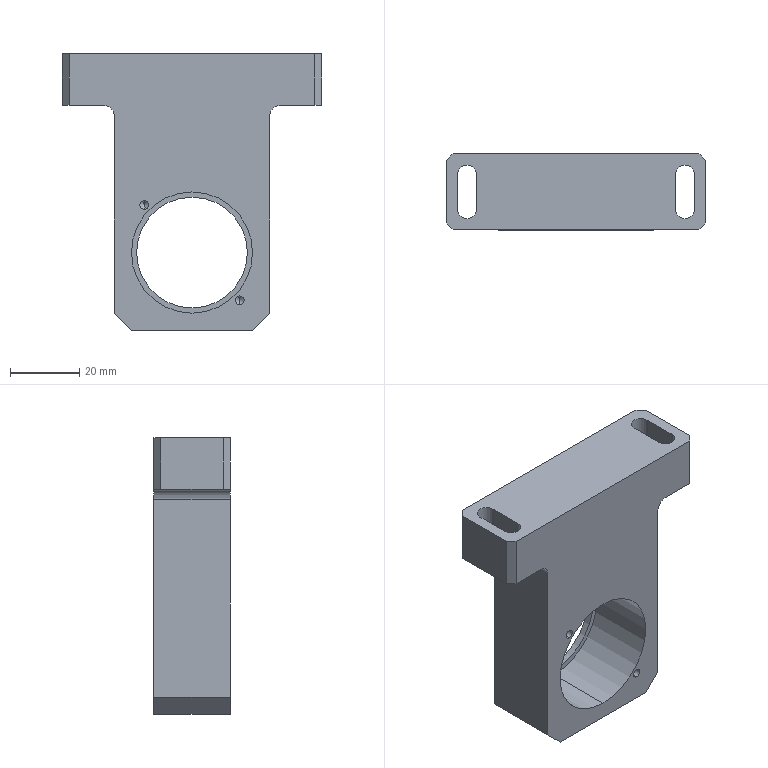Part | SolidWorks | features ICE 3, Chamfer 2, HoleWzd 2, CirPattern 1, Extrusion 1, Fillet 1 | 1 solid | 39 faces | box 75 x 22 x 80 mm | volume 65225 mm3 | plane 21 | cylinder 14 | cone 4 | commonest cylinder face diameters 2.5 x4 5.5 x4 6 x2 32 x2 35 x2
STEP:
#1=CARTESIAN_POINT('',(-13.789,-3.5,-2.461));
#2=VERTEX_POINT('',#1);
#3=CARTESIAN_POINT('',(-13.789,-3.5,-4.961));
#4=VERTEX_POINT('',#3);
#5=CARTESIAN_POINT('',(-13.789,-3.5,-3.711));
#6=DIRECTION('',(0.,-1.,0.));
#7=DIRECTION('',(0.,0.,-1.));
#8=AXIS2_PLACEMENT_3D('',#5,#6,#7);
#9=CIRCLE('',#8,1.25);
#10=EDGE_CURVE('',#2,#4,#9,.T.);
#11=ORIENTED_EDGE('',*,*,#10,.F.);
#12=CARTESIAN_POINT('',(-13.789,-11.,-2.461));
#13=VERTEX_POINT('',#12);
#14=CARTESIAN_POINT('',(-13.789,-11.,-2.461));
#15=DIRECTION('',(0.,-1.,0.));
#16=VECTOR('',#15,1000.);
#17=LINE('',#14,#16);
#18=EDGE_CURVE('',#2,#13,#17,.T.);
#19=ORIENTED_EDGE('',*,*,#18,.T.);
#20=CARTESIAN_POINT('',(-13.789,-11.,-4.961));
#21=VERTEX_POINT('',#20);
#22=CARTESIAN_POINT('',(-13.789,-11.,-3.711));
#23=DIRECTION('',(0.,-1.,0.));
#24=DIRECTION('',(0.,0.,-1.));
#25=AXIS2_PLACEMENT_3D('',#22,#23,#24);
#26=CIRCLE('',#25,1.25);
#27=EDGE_CURVE('',#13,#21,#26,.T.);
#28=ORIENTED_EDGE('',*,*,#27,.T.);
#29=CARTESIAN_POINT('',(-13.789,-11.,-4.961));
#30=DIRECTION('',(0.,-1.,0.));
#31=VECTOR('',#30,1000.);
#32=LINE('',#29,#31);
#33=EDGE_CURVE('',#4,#21,#32,.T.);
#34=ORIENTED_EDGE('',*,*,#33,.F.);
#35=EDGE_LOOP('',(#11,#19,#28,#34));
#36=FACE_OUTER_BOUND('',#35,.T.);
#37=CARTESIAN_POINT('',(-13.789,-11.,-3.711));
#38=DIRECTION('',(0.,-1.,0.));
#39=DIRECTION('',(0.,0.,-1.));
#40=AXIS2_PLACEMENT_3D('',#37,#38,#39);
#41=CYLINDRICAL_SURFACE('',#40,1.25);
#42=ADVANCED_FACE('',(#36),#41,.F.);
#43=CARTESIAN_POINT('',(-13.789,-2.749,-3.711));
#44=VERTEX_POINT('',#43);
#45=CARTESIAN_POINT('',(-13.789,-3.5,-4.961));
#46=DIRECTION('',(0.,-0.515,-0.8572));
#47=VECTOR('',#46,1000.);
#48=LINE('',#45,#47);
#49=EDGE_CURVE('',#44,#4,#48,.T.);
#50=ORIENTED_EDGE('',*,*,#49,.F.);
#51=CARTESIAN_POINT('',(-13.789,-3.5,-2.461));
#52=DIRECTION('',(0.,-0.515,0.8572));
#53=VECTOR('',#52,1000.);
#54=LINE('',#51,#53);
#55=EDGE_CURVE('',#44,#2,#54,.T.);
#56=ORIENTED_EDGE('',*,*,#55,.T.);
#57=ORIENTED_EDGE('',*,*,#10,.T.);
#58=EDGE_LOOP('',(#50,#56,#57));
#59=FACE_OUTER_BOUND('',#58,.T.);
#60=CARTESIAN_POINT('',(-13.789,-3.5,-3.711));
#61=DIRECTION('',(0.,-1.,0.));
#62=DIRECTION('',(0.,0.,-1.));
#63=AXIS2_PLACEMENT_3D('',#60,#61,#62);
#64=CONICAL_SURFACE('',#63,1.25,1.03);
#65=ADVANCED_FACE('',(#59),#64,.F.);
#66=CARTESIAN_POINT('',(13.789,-3.5,-30.039));
#67=VERTEX_POINT('',#66);
#68=CARTESIAN_POINT('',(13.789,-3.5,-32.539));
#69=VERTEX_POINT('',#68);
#70=CARTESIAN_POINT('',(13.789,-3.5,-31.289));
#71=DIRECTION('',(0.,-1.,0.));
#72=DIRECTION('',(0.,0.,-1.));
#73=AXIS2_PLACEMENT_3D('',#70,#71,#72);
#74=CIRCLE('',#73,1.25);
#75=EDGE_CURVE('',#67,#69,#74,.T.);
#76=ORIENTED_EDGE('',*,*,#75,.F.);
#77=CARTESIAN_POINT('',(13.789,-11.,-30.039));
#78=VERTEX_POINT('',#77);
#79=CARTESIAN_POINT('',(13.789,-11.,-30.039));
#80=DIRECTION('',(0.,-1.,0.));
#81=VECTOR('',#80,1000.);
#82=LINE('',#79,#81);
#83=EDGE_CURVE('',#67,#78,#82,.T.);
#84=ORIENTED_EDGE('',*,*,#83,.T.);
#85=CARTESIAN_POINT('',(13.789,-11.,-32.539));
#86=VERTEX_POINT('',#85);
#87=CARTESIAN_POINT('',(13.789,-11.,-31.289));
#88=DIRECTION('',(0.,-1.,0.));
#89=DIRECTION('',(0.,0.,-1.));
#90=AXIS2_PLACEMENT_3D('',#87,#88,#89);
#91=CIRCLE('',#90,1.25);
#92=EDGE_CURVE('',#78,#86,#91,.T.);
#93=ORIENTED_EDGE('',*,*,#92,.T.);
#94=CARTESIAN_POINT('',(13.789,-11.,-32.539));
#95=DIRECTION('',(0.,-1.,0.));
#96=VECTOR('',#95,1000.);
#97=LINE('',#94,#96);
#98=EDGE_CURVE('',#69,#86,#97,.T.);
#99=ORIENTED_EDGE('',*,*,#98,.F.);
#100=EDGE_LOOP('',(#76,#84,#93,#99));
#101=FACE_OUTER_BOUND('',#100,.T.);
#102=CARTESIAN_POINT('',(13.789,-11.,-31.289));
#103=DIRECTION('',(0.,-1.,0.));
#104=DIRECTION('',(0.,0.,-1.));
#105=AXIS2_PLACEMENT_3D('',#102,#103,#104);
#106=CYLINDRICAL_SURFACE('',#105,1.25);
#107=ADVANCED_FACE('',(#101),#106,.F.);
#108=CARTESIAN_POINT('',(13.789,-2.749,-31.289));
#109=VERTEX_POINT('',#108);
#110=CARTESIAN_POINT('',(13.789,-3.5,-32.539));
#111=DIRECTION('',(0.,-0.515,-0.8572));
#112=VECTOR('',#111,1000.);
#113=LINE('',#110,#112);
#114=EDGE_CURVE('',#109,#69,#113,.T.);
#115=ORIENTED_EDGE('',*,*,#114,.F.);
#116=CARTESIAN_POINT('',(13.789,-3.5,-30.039));
#117=DIRECTION('',(0.,-0.515,0.8572));
#118=VECTOR('',#117,1000.);
#119=LINE('',#116,#118);
#120=EDGE_CURVE('',#109,#67,#119,.T.);
#121=ORIENTED_EDGE('',*,*,#120,.T.);
#122=ORIENTED_EDGE('',*,*,#75,.T.);
#123=EDGE_LOOP('',(#115,#121,#122));
#124=FACE_OUTER_BOUND('',#123,.T.);
#125=CARTESIAN_POINT('',(13.789,-3.5,-31.289));
#126=DIRECTION('',(0.,-1.,0.));
#127=DIRECTION('',(0.,0.,-1.));
#128=AXIS2_PLACEMENT_3D('',#125,#126,#127);
#129=CONICAL_SURFACE('',#128,1.25,1.03);
#130=ADVANCED_FACE('',(#124),#129,.F.);
#131=CARTESIAN_POINT('',(0.,9.,-33.5));
#132=VERTEX_POINT('',#131);
#133=CARTESIAN_POINT('',(0.,9.,-1.5));
#134=VERTEX_POINT('',#133);
#135=CARTESIAN_POINT('',(0.,9.,-17.5));
#136=DIRECTION('',(0.,1.,0.));
#137=DIRECTION('',(0.,0.,1.));
#138=AXIS2_PLACEMENT_3D('',#135,#136,#137);
#139=CIRCLE('',#138,16.);
#140=EDGE_CURVE('',#132,#134,#139,.T.);
#141=ORIENTED_EDGE('',*,*,#140,.F.);
#142=CARTESIAN_POINT('',(0.,11.,-33.5));
#143=VERTEX_POINT('',#142);
#144=CARTESIAN_POINT('',(0.,9.,-33.5));
#145=DIRECTION('',(0.,1.,0.));
#146=VECTOR('',#145,1000.);
#147=LINE('',#144,#146);
#148=EDGE_CURVE('',#132,#143,#147,.T.);
#149=ORIENTED_EDGE('',*,*,#148,.T.);
#150=CARTESIAN_POINT('',(0.,11.,-1.5));
#151=VERTEX_POINT('',#150);
#152=CARTESIAN_POINT('',(0.,11.,-17.5));
#153=DIRECTION('',(0.,1.,0.));
#154=DIRECTION('',(0.,0.,1.));
#155=AXIS2_PLACEMENT_3D('',#152,#153,#154);
#156=CIRCLE('',#155,16.);
#157=EDGE_CURVE('',#143,#151,#156,.T.);
#158=ORIENTED_EDGE('',*,*,#157,.T.);
#159=CARTESIAN_POINT('',(0.,9.,-1.5));
#160=DIRECTION('',(0.,1.,0.));
#161=VECTOR('',#160,1000.);
#162=LINE('',#159,#161);
#163=EDGE_CURVE('',#134,#151,#162,.T.);
#164=ORIENTED_EDGE('',*,*,#163,.F.);
#165=EDGE_LOOP('',(#141,#149,#158,#164));
#166=FACE_OUTER_BOUND('',#165,.T.);
#167=CARTESIAN_POINT('',(0.,9.,-17.5));
#168=DIRECTION('',(0.,1.,0.));
#169=DIRECTION('',(0.,0.,1.));
#170=AXIS2_PLACEMENT_3D('',#167,#168,#169);
#171=CYLINDRICAL_SURFACE('',#170,16.);
#172=ADVANCED_FACE('',(#166),#171,.F.);
#173=CARTESIAN_POINT('',(0.,-11.,-35.));
#174=VERTEX_POINT('',#173);
#175=CARTESIAN_POINT('',(0.,-11.,0.));
#176=VERTEX_POINT('',#175);
#177=CARTESIAN_POINT('',(0.,-11.,-17.5));
#178=DIRECTION('',(0.,1.,0.));
#179=DIRECTION('',(0.,0.,1.));
#180=AXIS2_PLACEMENT_3D('',#177,#178,#179);
#181=CIRCLE('',#180,17.5);
#182=EDGE_CURVE('',#174,#176,#181,.T.);
#183=ORIENTED_EDGE('',*,*,#182,.F.);
#184=CARTESIAN_POINT('',(0.,9.,-35.));
#185=VERTEX_POINT('',#184);
#186=CARTESIAN_POINT('',(0.,-11.,-35.));
#187=DIRECTION('',(0.,1.,0.));
#188=VECTOR('',#187,1000.);
#189=LINE('',#186,#188);
#190=EDGE_CURVE('',#174,#185,#189,.T.);
#191=ORIENTED_EDGE('',*,*,#190,.T.);
#192=CARTESIAN_POINT('',(0.,9.,0.));
#193=VERTEX_POINT('',#192);
#194=CARTESIAN_POINT('',(0.,9.,-17.5));
#195=DIRECTION('',(0.,-1.,0.));
#196=DIRECTION('',(0.,0.,1.));
#197=AXIS2_PLACEMENT_3D('',#194,#195,#196);
#198=CIRCLE('',#197,17.5);
#199=EDGE_CURVE('',#193,#185,#198,.T.);
#200=ORIENTED_EDGE('',*,*,#199,.F.);
#201=CARTESIAN_POINT('',(0.,-11.,0.));
#202=DIRECTION('',(0.,1.,0.));
#203=VECTOR('',#202,1000.);
#204=LINE('',#201,#203);
#205=EDGE_CURVE('',#176,#193,#204,.T.);
#206=ORIENTED_EDGE('',*,*,#205,.F.);
#207=EDGE_LOOP('',(#183,#191,#200,#206));
#208=FACE_OUTER_BOUND('',#207,.T.);
#209=CARTESIAN_POINT('',(0.,-11.,-17.5));
#210=DIRECTION('',(0.,1.,0.));
#211=DIRECTION('',(0.,0.,1.));
#212=AXIS2_PLACEMENT_3D('',#209,#210,#211);
#213=CYLINDRICAL_SURFACE('',#212,17.5);
#214=ADVANCED_FACE('',(#208),#213,.F.);
#215=ORIENTED_EDGE('',*,*,#190,.F.);
#216=CARTESIAN_POINT('',(0.,-11.,-17.5));
#217=DIRECTION('',(0.,1.,0.));
#218=DIRECTION('',(0.,0.,1.));
#219=AXIS2_PLACEMENT_3D('',#216,#217,#218);
#220=CIRCLE('',#219,17.5);
#221=EDGE_CURVE('',#176,#174,#220,.T.);
#222=ORIENTED_EDGE('',*,*,#221,.F.);
#223=ORIENTED_EDGE('',*,*,#205,.T.);
#224=CARTESIAN_POINT('',(0.,9.,-17.5));
#225=DIRECTION('',(0.,-1.,0.));
#226=DIRECTION('',(0.,0.,1.));
#227=AXIS2_PLACEMENT_3D('',#224,#225,#226);
#228=CIRCLE('',#227,17.5);
#229=EDGE_CURVE('',#185,#193,#228,.T.);
#230=ORIENTED_EDGE('',*,*,#229,.F.);
#231=EDGE_LOOP('',(#215,#222,#223,#230));
#232=FACE_OUTER_BOUND('',#231,.T.);
#233=CARTESIAN_POINT('',(0.,-11.,-17.5));
#234=DIRECTION('',(0.,1.,0.));
#235=DIRECTION('',(0.,0.,1.));
#236=AXIS2_PLACEMENT_3D('',#233,#234,#235);
#237=CYLINDRICAL_SURFACE('',#236,17.5);
#238=ADVANCED_FACE('',(#232),#237,.F.);
#239=CARTESIAN_POINT('',(22.5,-11.,22.));
#240=VERTEX_POINT('',#239);
#241=CARTESIAN_POINT('',(22.5,-11.,-35.));
#242=VERTEX_POINT('',#241);
#243=CARTESIAN_POINT('',(22.5,-11.,40.));
#244=DIRECTION('',(0.,0.,-1.));
#245=VECTOR('',#244,1000.);
#246=LINE('',#243,#245);
#247=EDGE_CURVE('',#240,#242,#246,.T.);
#248=ORIENTED_EDGE('',*,*,#247,.T.);
#249=CARTESIAN_POINT('',(22.5,11.,-35.));
#250=VERTEX_POINT('',#249);
#251=CARTESIAN_POINT('',(22.5,11.,-35.));
#252=DIRECTION('',(0.,1.,0.));
#253=VECTOR('',#252,1000.);
#254=LINE('',#251,#253);
#255=EDGE_CURVE('',#242,#250,#254,.T.);
#256=ORIENTED_EDGE('',*,*,#255,.T.);
#257=CARTESIAN_POINT('',(22.5,11.,22.));
#258=VERTEX_POINT('',#257);
#259=CARTESIAN_POINT('',(22.5,11.,40.));
#260=DIRECTION('',(0.,0.,-1.));
#261=VECTOR('',#260,1000.);
#262=LINE('',#259,#261);
#263=EDGE_CURVE('',#258,#250,#262,.T.);
#264=ORIENTED_EDGE('',*,*,#263,.F.);
#265=CARTESIAN_POINT('',(22.5,11.,22.));
#266=DIRECTION('',(0.,-1.,0.));
#267=VECTOR('',#266,1000.);
#268=LINE('',#265,#267);
#269=EDGE_CURVE('',#258,#240,#268,.T.);
#270=ORIENTED_EDGE('',*,*,#269,.T.);
#271=EDGE_LOOP('',(#248,#256,#264,#270));
#272=FACE_OUTER_BOUND('',#271,.T.);
#273=CARTESIAN_POINT('',(22.5,11.,40.));
#274=DIRECTION('',(-1.,0.,0.));
#275=DIRECTION('',(0.,0.,1.));
#276=AXIS2_PLACEMENT_3D('',#273,#274,#275);
#277=PLANE('',#276);
#278=ADVANCED_FACE('',(#272),#277,.F.);
#279=CARTESIAN_POINT('',(17.5,-11.,-40.));
#280=VERTEX_POINT('',#279);
#281=CARTESIAN_POINT('',(-17.5,-11.,-40.));
#282=VERTEX_POINT('',#281);
#283=CARTESIAN_POINT('',(-22.5,-11.,-40.));
#284=DIRECTION('',(-1.,0.,0.));
#285=VECTOR('',#284,1000.);
#286=LINE('',#283,#285);
#287=EDGE_CURVE('',#280,#282,#286,.T.);
#288=ORIENTED_EDGE('',*,*,#287,.T.);
#289=CARTESIAN_POINT('',(-17.5,11.,-40.));
#290=VERTEX_POINT('',#289);
#291=CARTESIAN_POINT('',(-17.5,11.,-40.));
#292=DIRECTION('',(0.,1.,0.));
#293=VECTOR('',#292,1000.);
#294=LINE('',#291,#293);
#295=EDGE_CURVE('',#282,#290,#294,.T.);
#296=ORIENTED_EDGE('',*,*,#295,.T.);
#297=CARTESIAN_POINT('',(17.5,11.,-40.));
#298=VERTEX_POINT('',#297);
#299=CARTESIAN_POINT('',(-22.5,11.,-40.));
#300=DIRECTION('',(-1.,0.,0.));
#301=VECTOR('',#300,1000.);
#302=LINE('',#299,#301);
#303=EDGE_CURVE('',#298,#290,#302,.T.);
#304=ORIENTED_EDGE('',*,*,#303,.F.);
#305=CARTESIAN_POINT('',(17.5,11.,-40.));
#306=DIRECTION('',(0.,-1.,0.));
#307=VECTOR('',#306,1000.);
#308=LINE('',#305,#307);
#309=EDGE_CURVE('',#298,#280,#308,.T.);
#310=ORIENTED_EDGE('',*,*,#309,.T.);
#311=EDGE_LOOP('',(#288,#296,#304,#310));
#312=FACE_OUTER_BOUND('',#311,.T.);
#313=CARTESIAN_POINT('',(-22.5,11.,-40.));
#314=DIRECTION('',(0.,0.,1.));
#315=DIRECTION('',(1.,0.,0.));
#316=AXIS2_PLACEMENT_3D('',#313,#314,#315);
#317=PLANE('',#316);
#318=ADVANCED_FACE('',(#312),#317,.F.);
#319=CARTESIAN_POINT('',(-22.5,11.,-35.));
#320=VERTEX_POINT('',#319);
#321=CARTESIAN_POINT('',(-22.5,11.,22.));
#322=VERTEX_POINT('',#321);
#323=CARTESIAN_POINT('',(-22.5,11.,40.));
#324=DIRECTION('',(0.,0.,1.));
#325=VECTOR('',#324,1000.);
#326=LINE('',#323,#325);
#327=EDGE_CURVE('',#320,#322,#326,.T.);
#328=ORIENTED_EDGE('',*,*,#327,.F.);
#329=CARTESIAN_POINT('',(-22.5,-11.,-35.));
#330=VERTEX_POINT('',#329);
#331=CARTESIAN_POINT('',(-22.5,11.,-35.));
#332=DIRECTION('',(0.,-1.,0.));
#333=VECTOR('',#332,1000.);
#334=LINE('',#331,#333);
#335=EDGE_CURVE('',#320,#330,#334,.T.);
#336=ORIENTED_EDGE('',*,*,#335,.T.);
#337=CARTESIAN_POINT('',(-22.5,-11.,22.));
#338=VERTEX_POINT('',#337);
#339=CARTESIAN_POINT('',(-22.5,-11.,40.));
#340=DIRECTION('',(0.,0.,1.));
#341=VECTOR('',#340,1000.);
#342=LINE('',#339,#341);
#343=EDGE_CURVE('',#330,#338,#342,.T.);
#344=ORIENTED_EDGE('',*,*,#343,.T.);
#345=CARTESIAN_POINT('',(-22.5,11.,22.));
#346=DIRECTION('',(0.,1.,0.));
#347=VECTOR('',#346,1000.);
#348=LINE('',#345,#347);
#349=EDGE_CURVE('',#338,#322,#348,.T.);
#350=ORIENTED_EDGE('',*,*,#349,.T.);
#351=EDGE_LOOP('',(#328,#336,#344,#350));
#352=FACE_OUTER_BOUND('',#351,.T.);
#353=CARTESIAN_POINT('',(-22.5,11.,40.));
#354=DIRECTION('',(1.,0.,0.));
#355=DIRECTION('',(0.,0.,-1.));
#356=AXIS2_PLACEMENT_3D('',#353,#354,#355);
#357=PLANE('',#356);
#358=ADVANCED_FACE('',(#352),#357,.F.);
#359=CARTESIAN_POINT('',(28.75,-5.,40.));
#360=VERTEX_POINT('',#359);
#361=CARTESIAN_POINT('',(28.75,5.,40.));
#362=VERTEX_POINT('',#361);
#363=CARTESIAN_POINT('',(28.75,-5.,40.));
#364=DIRECTION('',(0.,1.,0.));
#365=VECTOR('',#364,1000.);
#366=LINE('',#363,#365);
#367=EDGE_CURVE('',#360,#362,#366,.T.);
#368=ORIENTED_EDGE('',*,*,#367,.T.);
#369=CARTESIAN_POINT('',(34.25,5.,40.));
#370=VERTEX_POINT('',#369);
#371=CARTESIAN_POINT('',(31.5,5.,40.));
#372=DIRECTION('',(0.,0.,-1.));
#373=DIRECTION('',(-1.,0.,0.));
#374=AXIS2_PLACEMENT_3D('',#371,#372,#373);
#375=CIRCLE('',#374,2.75);
#376=EDGE_CURVE('',#362,#370,#375,.T.);
#377=ORIENTED_EDGE('',*,*,#376,.T.);
#378=CARTESIAN_POINT('',(34.25,-5.,40.));
#379=VERTEX_POINT('',#378);
#380=CARTESIAN_POINT('',(34.25,-5.,40.));
#381=DIRECTION('',(0.,1.,0.));
#382=VECTOR('',#381,1000.);
#383=LINE('',#380,#382);
#384=EDGE_CURVE('',#379,#370,#383,.T.);
#385=ORIENTED_EDGE('',*,*,#384,.F.);
#386=CARTESIAN_POINT('',(31.5,-5.,40.));
#387=DIRECTION('',(0.,0.,-1.));
#388=DIRECTION('',(-1.,0.,0.));
#389=AXIS2_PLACEMENT_3D('',#386,#387,#388);
#390=CIRCLE('',#389,2.75);
#391=EDGE_CURVE('',#379,#360,#390,.T.);
#392=ORIENTED_EDGE('',*,*,#391,.T.);
#393=EDGE_LOOP('',(#368,#377,#385,#392));
#394=FACE_BOUND('',#393,.T.);
#395=CARTESIAN_POINT('',(-34.25,-5.,40.));
#396=VERTEX_POINT('',#395);
#397=CARTESIAN_POINT('',(-34.25,5.,40.));
#398=VERTEX_POINT('',#397);
#399=CARTESIAN_POINT('',(-34.25,-5.,40.));
#400=DIRECTION('',(0.,1.,0.));
#401=VECTOR('',#400,1000.);
#402=LINE('',#399,#401);
#403=EDGE_CURVE('',#396,#398,#402,.T.);
#404=ORIENTED_EDGE('',*,*,#403,.T.);
#405=CARTESIAN_POINT('',(-28.75,5.,40.));
#406=VERTEX_POINT('',#405);
#407=CARTESIAN_POINT('',(-31.5,5.,40.));
#408=DIRECTION('',(0.,0.,-1.));
#409=DIRECTION('',(-1.,0.,0.));
#410=AXIS2_PLACEMENT_3D('',#407,#408,#409);
#411=CIRCLE('',#410,2.75);
#412=EDGE_CURVE('',#398,#406,#411,.T.);
#413=ORIENTED_EDGE('',*,*,#412,.T.);
#414=CARTESIAN_POINT('',(-28.75,-5.,40.));
#415=VERTEX_POINT('',#414);
#416=CARTESIAN_POINT('',(-28.75,-5.,40.));
#417=DIRECTION('',(0.,1.,0.));
#418=VECTOR('',#417,1000.);
#419=LINE('',#416,#418);
#420=EDGE_CURVE('',#415,#406,#419,.T.);
#421=ORIENTED_EDGE('',*,*,#420,.F.);
#422=CARTESIAN_POINT('',(-31.5,-5.,40.));
#423=DIRECTION('',(0.,0.,-1.));
#424=DIRECTION('',(-1.,0.,0.));
#425=AXIS2_PLACEMENT_3D('',#422,#423,#424);
#426=CIRCLE('',#425,2.75);
#427=EDGE_CURVE('',#415,#396,#426,.T.);
#428=ORIENTED_EDGE('',*,*,#427,.T.);
#429=EDGE_LOOP('',(#404,#413,#421,#428));
#430=FACE_BOUND('',#429,.T.);
#431=CARTESIAN_POINT('',(-37.5,-9.,40.));
#432=VERTEX_POINT('',#431);
#433=CARTESIAN_POINT('',(-37.5,9.,40.));
#434=VERTEX_POINT('',#433);
#435=CARTESIAN_POINT('',(-37.5,-32.213,40.));
#436=DIRECTION('',(0.,1.,0.));
#437=VECTOR('',#436,1000.);
#438=LINE('',#435,#437);
#439=EDGE_CURVE('',#432,#434,#438,.T.);
#440=ORIENTED_EDGE('',*,*,#439,.F.);
#441=CARTESIAN_POINT('',(-35.5,-11.,40.));
#442=VERTEX_POINT('',#441);
#443=CARTESIAN_POINT('',(-37.5,-9.,40.));
#444=DIRECTION('',(0.7071,-0.7071,0.));
#445=VECTOR('',#444,1000.);
#446=LINE('',#443,#445);
#447=EDGE_CURVE('',#432,#442,#446,.T.);
#448=ORIENTED_EDGE('',*,*,#447,.T.);
#449=CARTESIAN_POINT('',(35.5,-11.,40.));
#450=VERTEX_POINT('',#449);
#451=CARTESIAN_POINT('',(-22.5,-11.,40.));
#452=DIRECTION('',(1.,0.,0.));
#453=VECTOR('',#452,1000.);
#454=LINE('',#451,#453);
#455=EDGE_CURVE('',#442,#450,#454,.T.);
#456=ORIENTED_EDGE('',*,*,#455,.T.);
#457=CARTESIAN_POINT('',(37.5,-9.,40.));
#458=VERTEX_POINT('',#457);
#459=CARTESIAN_POINT('',(37.5,-9.,40.));
#460=DIRECTION('',(0.7071,0.7071,0.));
#461=VECTOR('',#460,1000.);
#462=LINE('',#459,#461);
#463=EDGE_CURVE('',#450,#458,#462,.T.);
#464=ORIENTED_EDGE('',*,*,#463,.T.);
#465=CARTESIAN_POINT('',(37.5,9.,40.));
#466=VERTEX_POINT('',#465);
#467=CARTESIAN_POINT('',(37.5,-32.213,40.));
#468=DIRECTION('',(0.,1.,0.));
#469=VECTOR('',#468,1000.);
#470=LINE('',#467,#469);
#471=EDGE_CURVE('',#458,#466,#470,.T.);
#472=ORIENTED_EDGE('',*,*,#471,.T.);
#473=CARTESIAN_POINT('',(35.5,11.,40.));
#474=VERTEX_POINT('',#473);
#475=CARTESIAN_POINT('',(35.5,11.,40.));
#476=DIRECTION('',(-0.7071,0.7071,0.));
#477=VECTOR('',#476,1000.);
#478=LINE('',#475,#477);
#479=EDGE_CURVE('',#466,#474,#478,.T.);
#480=ORIENTED_EDGE('',*,*,#479,.T.);
#481=CARTESIAN_POINT('',(-35.5,11.,40.));
#482=VERTEX_POINT('',#481);
#483=CARTESIAN_POINT('',(-22.5,11.,40.));
#484=DIRECTION('',(1.,0.,0.));
#485=VECTOR('',#484,1000.);
#486=LINE('',#483,#485);
#487=EDGE_CURVE('',#482,#474,#486,.T.);
#488=ORIENTED_EDGE('',*,*,#487,.F.);
#489=CARTESIAN_POINT('',(-35.5,11.,40.));
#490=DIRECTION('',(-0.7071,-0.7071,0.));
#491=VECTOR('',#490,1000.);
#492=LINE('',#489,#491);
#493=EDGE_CURVE('',#482,#434,#492,.T.);
#494=ORIENTED_EDGE('',*,*,#493,.T.);
#495=EDGE_LOOP('',(#440,#448,#456,#464,#472,#480,#488,#494));
#496=FACE_OUTER_BOUND('',#495,.T.);
#497=CARTESIAN_POINT('',(-22.5,11.,40.));
#498=DIRECTION('',(0.,0.,-1.));
#499=DIRECTION('',(-1.,0.,0.));
#500=AXIS2_PLACEMENT_3D('',#497,#498,#499);
#501=PLANE('',#500);
#502=ADVANCED_FACE('',(#394,#430,#496),#501,.F.);
#503=CARTESIAN_POINT('',(-25.5,11.,25.));
#504=VERTEX_POINT('',#503);
#505=CARTESIAN_POINT('',(-35.5,11.,25.));
#506=VERTEX_POINT('',#505);
#507=CARTESIAN_POINT('',(-22.5,11.,25.));
#508=DIRECTION('',(-1.,0.,0.));
#509=VECTOR('',#508,1000.);
#510=LINE('',#507,#509);
#511=EDGE_CURVE('',#504,#506,#510,.T.);
#512=ORIENTED_EDGE('',*,*,#511,.T.);
#513=CARTESIAN_POINT('',(-35.5,11.,40.));
#514=DIRECTION('',(0.,0.,1.));
#515=VECTOR('',#514,1000.);
#516=LINE('',#513,#515);
#517=EDGE_CURVE('',#506,#482,#516,.T.);
#518=ORIENTED_EDGE('',*,*,#517,.T.);
#519=ORIENTED_EDGE('',*,*,#487,.T.);
#520=CARTESIAN_POINT('',(35.5,11.,25.));
#521=VERTEX_POINT('',#520);
#522=CARTESIAN_POINT('',(35.5,11.,25.));
#523=DIRECTION('',(0.,0.,-1.));
#524=VECTOR('',#523,1000.);
#525=LINE('',#522,#524);
#526=EDGE_CURVE('',#474,#521,#525,.T.);
#527=ORIENTED_EDGE('',*,*,#526,.T.);
#528=CARTESIAN_POINT('',(25.5,11.,25.));
#529=VERTEX_POINT('',#528);
#530=CARTESIAN_POINT('',(22.5,11.,25.));
#531=DIRECTION('',(-1.,0.,0.));
#532=VECTOR('',#531,1000.);
#533=LINE('',#530,#532);
#534=EDGE_CURVE('',#521,#529,#533,.T.);
#535=ORIENTED_EDGE('',*,*,#534,.T.);
#536=CARTESIAN_POINT('',(25.5,11.,22.));
#537=DIRECTION('',(0.,-1.,0.));
#538=DIRECTION('',(0.,0.,-1.));
#539=AXIS2_PLACEMENT_3D('',#536,#537,#538);
#540=CIRCLE('',#539,3.);
#541=EDGE_CURVE('',#529,#258,#540,.T.);
#542=ORIENTED_EDGE('',*,*,#541,.T.);
#543=ORIENTED_EDGE('',*,*,#263,.T.);
#544=CARTESIAN_POINT('',(17.5,11.,-40.));
#545=DIRECTION('',(-0.7071,0.,-0.7071));
#546=VECTOR('',#545,1000.);
#547=LINE('',#544,#546);
#548=EDGE_CURVE('',#250,#298,#547,.T.);
#549=ORIENTED_EDGE('',*,*,#548,.T.);
#550=ORIENTED_EDGE('',*,*,#303,.T.);
#551=CARTESIAN_POINT('',(-22.5,11.,-35.));
#552=DIRECTION('',(-0.7071,0.,0.7071));
#553=VECTOR('',#552,1000.);
#554=LINE('',#551,#553);
#555=EDGE_CURVE('',#290,#320,#554,.T.);
#556=ORIENTED_EDGE('',*,*,#555,.T.);
#557=ORIENTED_EDGE('',*,*,#327,.T.);
#558=CARTESIAN_POINT('',(-25.5,11.,22.));
#559=DIRECTION('',(0.,-1.,0.));
#560=DIRECTION('',(0.,0.,-1.));
#561=AXIS2_PLACEMENT_3D('',#558,#559,#560);
#562=CIRCLE('',#561,3.);
#563=EDGE_CURVE('',#322,#504,#562,.T.);
#564=ORIENTED_EDGE('',*,*,#563,.T.);
#565=EDGE_LOOP('',(#512,#518,#519,#527,#535,#542,#543,#549,#550,#556,#557,#564));
#566=FACE_OUTER_BOUND('',#565,.T.);
#567=CARTESIAN_POINT('',(0.,11.,-17.5));
#568=DIRECTION('',(0.,1.,0.));
#569=DIRECTION('',(0.,0.,1.));
#570=AXIS2_PLACEMENT_3D('',#567,#568,#569);
#571=CIRCLE('',#570,16.);
#572=EDGE_CURVE('',#151,#143,#571,.T.);
#573=ORIENTED_EDGE('',*,*,#572,.F.);
#574=ORIENTED_EDGE('',*,*,#157,.F.);
#575=EDGE_LOOP('',(#573,#574));
#576=FACE_BOUND('',#575,.T.);
#577=CARTESIAN_POINT('',(0.,11.,0.));
#578=DIRECTION('',(0.,-1.,0.));
#579=DIRECTION('',(0.,0.,-1.));
#580=AXIS2_PLACEMENT_3D('',#577,#578,#579);
#581=PLANE('',#580);
#582=ADVANCED_FACE('',(#566,#576),#581,.F.);
#583=CARTESIAN_POINT('',(-13.789,-11.,-3.711));
#584=DIRECTION('',(0.,-1.,0.));
#585=DIRECTION('',(0.,0.,-1.));
#586=AXIS2_PLACEMENT_3D('',#583,#584,#585);
#587=CIRCLE('',#586,1.25);
#588=EDGE_CURVE('',#21,#13,#587,.T.);
#589=ORIENTED_EDGE('',*,*,#588,.F.);
#590=ORIENTED_EDGE('',*,*,#27,.F.);
#591=EDGE_LOOP('',(#589,#590));
#592=FACE_BOUND('',#591,.T.);
#593=CARTESIAN_POINT('',(13.789,-11.,-31.289));
#594=DIRECTION('',(0.,-1.,0.));
#595=DIRECTION('',(0.,0.,-1.));
#596=AXIS2_PLACEMENT_3D('',#593,#594,#595);
#597=CIRCLE('',#596,1.25);
#598=EDGE_CURVE('',#86,#78,#597,.T.);
#599=ORIENTED_EDGE('',*,*,#598,.F.);
#600=ORIENTED_EDGE('',*,*,#92,.F.);
#601=EDGE_LOOP('',(#599,#600));
#602=FACE_BOUND('',#601,.T.);
#603=ORIENTED_EDGE('',*,*,#221,.T.);
#604=ORIENTED_EDGE('',*,*,#182,.T.);
#605=EDGE_LOOP('',(#603,#604));
#606=FACE_BOUND('',#605,.T.);
#607=ORIENTED_EDGE('',*,*,#455,.F.);
#608=CARTESIAN_POINT('',(-35.5,-11.,25.));
#609=VERTEX_POINT('',#608);
#610=CARTESIAN_POINT('',(-35.5,-11.,0.));
#611=DIRECTION('',(0.,0.,-1.));
#612=VECTOR('',#611,1000.);
#613=LINE('',#610,#612);
#614=EDGE_CURVE('',#442,#609,#613,.T.);
#615=ORIENTED_EDGE('',*,*,#614,.T.);
#616=CARTESIAN_POINT('',(-25.5,-11.,25.));
#617=VERTEX_POINT('',#616);
#618=CARTESIAN_POINT('',(-22.5,-11.,25.));
#619=DIRECTION('',(-1.,0.,0.));
#620=VECTOR('',#619,1000.);
#621=LINE('',#618,#620);
#622=EDGE_CURVE('',#617,#609,#621,.T.);
#623=ORIENTED_EDGE('',*,*,#622,.F.);
#624=CARTESIAN_POINT('',(-25.5,-11.,22.));
#625=DIRECTION('',(0.,1.,0.));
#626=DIRECTION('',(0.,0.,-1.));
#627=AXIS2_PLACEMENT_3D('',#624,#625,#626);
#628=CIRCLE('',#627,3.);
#629=EDGE_CURVE('',#617,#338,#628,.T.);
#630=ORIENTED_EDGE('',*,*,#629,.T.);
#631=ORIENTED_EDGE('',*,*,#343,.F.);
#632=CARTESIAN_POINT('',(-28.75,-11.,-28.75));
#633=DIRECTION('',(0.7071,0.,-0.7071));
#634=VECTOR('',#633,1000.);
#635=LINE('',#632,#634);
#636=EDGE_CURVE('',#330,#282,#635,.T.);
#637=ORIENTED_EDGE('',*,*,#636,.T.);
#638=ORIENTED_EDGE('',*,*,#287,.F.);
#639=CARTESIAN_POINT('',(28.75,-11.,-28.75));
#640=DIRECTION('',(0.7071,0.,0.7071));
#641=VECTOR('',#640,1000.);
#642=LINE('',#639,#641);
#643=EDGE_CURVE('',#280,#242,#642,.T.);
#644=ORIENTED_EDGE('',*,*,#643,.T.);
#645=ORIENTED_EDGE('',*,*,#247,.F.);
#646=CARTESIAN_POINT('',(25.5,-11.,25.));
#647=VERTEX_POINT('',#646);
#648=CARTESIAN_POINT('',(25.5,-11.,22.));
#649=DIRECTION('',(0.,1.,0.));
#650=DIRECTION('',(0.,0.,-1.));
#651=AXIS2_PLACEMENT_3D('',#648,#649,#650);
#652=CIRCLE('',#651,3.);
#653=EDGE_CURVE('',#240,#647,#652,.T.);
#654=ORIENTED_EDGE('',*,*,#653,.T.);
#655=CARTESIAN_POINT('',(35.5,-11.,25.));
#656=VERTEX_POINT('',#655);
#657=CARTESIAN_POINT('',(22.5,-11.,25.));
#658=DIRECTION('',(-1.,0.,0.));
#659=VECTOR('',#658,1000.);
#660=LINE('',#657,#659);
#661=EDGE_CURVE('',#656,#647,#660,.T.);
#662=ORIENTED_EDGE('',*,*,#661,.F.);
#663=CARTESIAN_POINT('',(35.5,-11.,0.));
#664=DIRECTION('',(0.,0.,1.));
#665=VECTOR('',#664,1000.);
#666=LINE('',#663,#665);
#667=EDGE_CURVE('',#656,#450,#666,.T.);
#668=ORIENTED_EDGE('',*,*,#667,.T.);
#669=EDGE_LOOP('',(#607,#615,#623,#630,#631,#637,#638,#644,#645,#654,#662,#668));
#670=FACE_OUTER_BOUND('',#669,.T.);
#671=CARTESIAN_POINT('',(0.,-11.,0.));
#672=DIRECTION('',(0.,-1.,0.));
#673=DIRECTION('',(0.,0.,-1.));
#674=AXIS2_PLACEMENT_3D('',#671,#672,#673);
#675=PLANE('',#674);
#676=ADVANCED_FACE('',(#592,#602,#606,#670),#675,.T.);
#677=CARTESIAN_POINT('',(-34.25,-5.,25.));
#678=VERTEX_POINT('',#677);
#679=CARTESIAN_POINT('',(-34.25,5.,25.));
#680=VERTEX_POINT('',#679);
#681=CARTESIAN_POINT('',(-34.25,-5.,25.));
#682=DIRECTION('',(0.,1.,0.));
#683=VECTOR('',#682,1000.);
#684=LINE('',#681,#683);
#685=EDGE_CURVE('',#678,#680,#684,.T.);
#686=ORIENTED_EDGE('',*,*,#685,.F.);
#687=CARTESIAN_POINT('',(-28.75,-5.,25.));
#688=VERTEX_POINT('',#687);
#689=CARTESIAN_POINT('',(-31.5,-5.,25.));
#690=DIRECTION('',(0.,0.,-1.));
#691=DIRECTION('',(-1.,0.,0.));
#692=AXIS2_PLACEMENT_3D('',#689,#690,#691);
#693=CIRCLE('',#692,2.75);
#694=EDGE_CURVE('',#688,#678,#693,.T.);
#695=ORIENTED_EDGE('',*,*,#694,.F.);
#696=CARTESIAN_POINT('',(-28.75,5.,25.));
#697=VERTEX_POINT('',#696);
#698=CARTESIAN_POINT('',(-28.75,-5.,25.));
#699=DIRECTION('',(0.,1.,0.));
#700=VECTOR('',#699,1000.);
#701=LINE('',#698,#700);
#702=EDGE_CURVE('',#688,#697,#701,.T.);
#703=ORIENTED_EDGE('',*,*,#702,.T.);
#704=CARTESIAN_POINT('',(-31.5,5.,25.));
#705=DIRECTION('',(0.,0.,-1.));
#706=DIRECTION('',(-1.,0.,0.));
#707=AXIS2_PLACEMENT_3D('',#704,#705,#706);
#708=CIRCLE('',#707,2.75);
#709=EDGE_CURVE('',#680,#697,#708,.T.);
#710=ORIENTED_EDGE('',*,*,#709,.F.);
#711=EDGE_LOOP('',(#686,#695,#703,#710));
#712=FACE_BOUND('',#711,.T.);
#713=ORIENTED_EDGE('',*,*,#622,.T.);
#714=CARTESIAN_POINT('',(-37.5,-9.,25.));
#715=VERTEX_POINT('',#714);
#716=CARTESIAN_POINT('',(-18.393,-28.107,25.));
#717=DIRECTION('',(-0.7071,0.7071,0.));
#718=VECTOR('',#717,1000.);
#719=LINE('',#716,#718);
#720=EDGE_CURVE('',#609,#715,#719,.T.);
#721=ORIENTED_EDGE('',*,*,#720,.T.);
#722=CARTESIAN_POINT('',(-37.5,9.,25.));
#723=VERTEX_POINT('',#722);
#724=CARTESIAN_POINT('',(-37.5,-32.213,25.));
#725=DIRECTION('',(0.,1.,0.));
#726=VECTOR('',#725,1000.);
#727=LINE('',#724,#726);
#728=EDGE_CURVE('',#715,#723,#727,.T.);
#729=ORIENTED_EDGE('',*,*,#728,.T.);
#730=CARTESIAN_POINT('',(-50.607,-4.107,25.));
#731=DIRECTION('',(0.7071,0.7071,0.));
#732=VECTOR('',#731,1000.);
#733=LINE('',#730,#732);
#734=EDGE_CURVE('',#723,#506,#733,.T.);
#735=ORIENTED_EDGE('',*,*,#734,.T.);
#736=ORIENTED_EDGE('',*,*,#511,.F.);
#737=CARTESIAN_POINT('',(-25.5,-32.213,25.));
#738=DIRECTION('',(0.,-1.,0.));
#739=VECTOR('',#738,1000.);
#740=LINE('',#737,#739);
#741=EDGE_CURVE('',#504,#617,#740,.T.);
#742=ORIENTED_EDGE('',*,*,#741,.T.);
#743=EDGE_LOOP('',(#713,#721,#729,#735,#736,#742));
#744=FACE_OUTER_BOUND('',#743,.T.);
#745=CARTESIAN_POINT('',(-22.5,-32.213,25.));
#746=DIRECTION('',(0.,0.,-1.));
#747=DIRECTION('',(-1.,0.,0.));
#748=AXIS2_PLACEMENT_3D('',#745,#746,#747);
#749=PLANE('',#748);
#750=ADVANCED_FACE('',(#712,#744),#749,.T.);
#751=ORIENTED_EDGE('',*,*,#728,.F.);
#752=CARTESIAN_POINT('',(-37.5,-9.,40.));
#753=DIRECTION('',(0.,0.,1.));
#754=VECTOR('',#753,1000.);
#755=LINE('',#752,#754);
#756=EDGE_CURVE('',#715,#432,#755,.T.);
#757=ORIENTED_EDGE('',*,*,#756,.T.);
#758=ORIENTED_EDGE('',*,*,#439,.T.);
#759=CARTESIAN_POINT('',(-37.5,9.,25.));
#760=DIRECTION('',(0.,0.,-1.));
#761=VECTOR('',#760,1000.);
#762=LINE('',#759,#761);
#763=EDGE_CURVE('',#434,#723,#762,.T.);
#764=ORIENTED_EDGE('',*,*,#763,.T.);
#765=EDGE_LOOP('',(#751,#757,#758,#764));
#766=FACE_OUTER_BOUND('',#765,.T.);
#767=CARTESIAN_POINT('',(-37.5,-32.213,40.));
#768=DIRECTION('',(-1.,0.,0.));
#769=DIRECTION('',(0.,0.,1.));
#770=AXIS2_PLACEMENT_3D('',#767,#768,#769);
#771=PLANE('',#770);
#772=ADVANCED_FACE('',(#766),#771,.T.);
#773=CARTESIAN_POINT('',(37.5,-9.,25.));
#774=VERTEX_POINT('',#773);
#775=CARTESIAN_POINT('',(37.5,9.,25.));
#776=VERTEX_POINT('',#775);
#777=CARTESIAN_POINT('',(37.5,-32.213,25.));
#778=DIRECTION('',(0.,1.,0.));
#779=VECTOR('',#778,1000.);
#780=LINE('',#777,#779);
#781=EDGE_CURVE('',#774,#776,#780,.T.);
#782=ORIENTED_EDGE('',*,*,#781,.T.);
#783=CARTESIAN_POINT('',(37.5,9.,40.));
#784=DIRECTION('',(0.,0.,1.));
#785=VECTOR('',#784,1000.);
#786=LINE('',#783,#785);
#787=EDGE_CURVE('',#776,#466,#786,.T.);
#788=ORIENTED_EDGE('',*,*,#787,.T.);
#789=ORIENTED_EDGE('',*,*,#471,.F.);
#790=CARTESIAN_POINT('',(37.5,-9.,40.));
#791=DIRECTION('',(0.,0.,-1.));
#792=VECTOR('',#791,1000.);
#793=LINE('',#790,#792);
#794=EDGE_CURVE('',#458,#774,#793,.T.);
#795=ORIENTED_EDGE('',*,*,#794,.T.);
#796=EDGE_LOOP('',(#782,#788,#789,#795));
#797=FACE_OUTER_BOUND('',#796,.T.);
#798=CARTESIAN_POINT('',(37.5,-32.213,40.));
#799=DIRECTION('',(1.,0.,0.));
#800=DIRECTION('',(0.,0.,-1.));
#801=AXIS2_PLACEMENT_3D('',#798,#799,#800);
#802=PLANE('',#801);
#803=ADVANCED_FACE('',(#797),#802,.T.);
#804=CARTESIAN_POINT('',(28.75,5.,25.));
#805=VERTEX_POINT('',#804);
#806=CARTESIAN_POINT('',(34.25,5.,25.));
#807=VERTEX_POINT('',#806);
#808=CARTESIAN_POINT('',(31.5,5.,25.));
#809=DIRECTION('',(0.,0.,-1.));
#810=DIRECTION('',(-1.,0.,0.));
#811=AXIS2_PLACEMENT_3D('',#808,#809,#810);
#812=CIRCLE('',#811,2.75);
#813=EDGE_CURVE('',#805,#807,#812,.T.);
#814=ORIENTED_EDGE('',*,*,#813,.F.);
#815=CARTESIAN_POINT('',(28.75,-5.,25.));
#816=VERTEX_POINT('',#815);
#817=CARTESIAN_POINT('',(28.75,-5.,25.));
#818=DIRECTION('',(0.,1.,0.));
#819=VECTOR('',#818,1000.);
#820=LINE('',#817,#819);
#821=EDGE_CURVE('',#816,#805,#820,.T.);
#822=ORIENTED_EDGE('',*,*,#821,.F.);
#823=CARTESIAN_POINT('',(34.25,-5.,25.));
#824=VERTEX_POINT('',#823);
#825=CARTESIAN_POINT('',(31.5,-5.,25.));
#826=DIRECTION('',(0.,0.,-1.));
#827=DIRECTION('',(-1.,0.,0.));
#828=AXIS2_PLACEMENT_3D('',#825,#826,#827);
#829=CIRCLE('',#828,2.75);
#830=EDGE_CURVE('',#824,#816,#829,.T.);
#831=ORIENTED_EDGE('',*,*,#830,.F.);
#832=CARTESIAN_POINT('',(34.25,-5.,25.));
#833=DIRECTION('',(0.,1.,0.));
#834=VECTOR('',#833,1000.);
#835=LINE('',#832,#834);
#836=EDGE_CURVE('',#824,#807,#835,.T.);
#837=ORIENTED_EDGE('',*,*,#836,.T.);
#838=EDGE_LOOP('',(#814,#822,#831,#837));
#839=FACE_BOUND('',#838,.T.);
#840=ORIENTED_EDGE('',*,*,#534,.F.);
#841=CARTESIAN_POINT('',(50.607,-4.107,25.));
#842=DIRECTION('',(0.7071,-0.7071,0.));
#843=VECTOR('',#842,1000.);
#844=LINE('',#841,#843);
#845=EDGE_CURVE('',#521,#776,#844,.T.);
#846=ORIENTED_EDGE('',*,*,#845,.T.);
#847=ORIENTED_EDGE('',*,*,#781,.F.);
#848=CARTESIAN_POINT('',(18.393,-28.107,25.));
#849=DIRECTION('',(-0.7071,-0.7071,0.));
#850=VECTOR('',#849,1000.);
#851=LINE('',#848,#850);
#852=EDGE_CURVE('',#774,#656,#851,.T.);
#853=ORIENTED_EDGE('',*,*,#852,.T.);
#854=ORIENTED_EDGE('',*,*,#661,.T.);
#855=CARTESIAN_POINT('',(25.5,-32.213,25.));
#856=DIRECTION('',(0.,1.,0.));
#857=VECTOR('',#856,1000.);
#858=LINE('',#855,#857);
#859=EDGE_CURVE('',#647,#529,#858,.T.);
#860=ORIENTED_EDGE('',*,*,#859,.T.);
#861=EDGE_LOOP('',(#840,#846,#847,#853,#854,#860));
#862=FACE_OUTER_BOUND('',#861,.T.);
#863=CARTESIAN_POINT('',(22.5,-32.213,25.));
#864=DIRECTION('',(0.,0.,-1.));
#865=DIRECTION('',(-1.,0.,0.));
#866=AXIS2_PLACEMENT_3D('',#863,#864,#865);
#867=PLANE('',#866);
#868=ADVANCED_FACE('',(#839,#862),#867,.T.);
#869=ORIENTED_EDGE('',*,*,#653,.F.);
#870=ORIENTED_EDGE('',*,*,#269,.F.);
#871=ORIENTED_EDGE('',*,*,#541,.F.);
#872=ORIENTED_EDGE('',*,*,#859,.F.);
#873=EDGE_LOOP('',(#869,#870,#871,#872));
#874=FACE_OUTER_BOUND('',#873,.T.);
#875=CARTESIAN_POINT('',(25.5,-32.213,22.));
#876=DIRECTION('',(0.,1.,0.));
#877=DIRECTION('',(0.,0.,1.));
#878=AXIS2_PLACEMENT_3D('',#875,#876,#877);
#879=CYLINDRICAL_SURFACE('',#878,3.);
#880=ADVANCED_FACE('',(#874),#879,.F.);
#881=ORIENTED_EDGE('',*,*,#629,.F.);
#882=ORIENTED_EDGE('',*,*,#741,.F.);
#883=ORIENTED_EDGE('',*,*,#563,.F.);
#884=ORIENTED_EDGE('',*,*,#349,.F.);
#885=EDGE_LOOP('',(#881,#882,#883,#884));
#886=FACE_OUTER_BOUND('',#885,.T.);
#887=CARTESIAN_POINT('',(-25.5,11.,22.));
#888=DIRECTION('',(0.,1.,0.));
#889=DIRECTION('',(0.,0.,1.));
#890=AXIS2_PLACEMENT_3D('',#887,#888,#889);
#891=CYLINDRICAL_SURFACE('',#890,3.);
#892=ADVANCED_FACE('',(#886),#891,.F.);
#893=ORIENTED_EDGE('',*,*,#555,.F.);
#894=ORIENTED_EDGE('',*,*,#295,.F.);
#895=ORIENTED_EDGE('',*,*,#636,.F.);
#896=ORIENTED_EDGE('',*,*,#335,.F.);
#897=EDGE_LOOP('',(#893,#894,#895,#896));
#898=FACE_OUTER_BOUND('',#897,.T.);
#899=CARTESIAN_POINT('',(-22.5,11.,-35.));
#900=DIRECTION('',(0.7071,0.,0.7071));
#901=DIRECTION('',(0.,-1.,0.));
#902=AXIS2_PLACEMENT_3D('',#899,#900,#901);
#903=PLANE('',#902);
#904=ADVANCED_FACE('',(#898),#903,.F.);
#905=ORIENTED_EDGE('',*,*,#548,.F.);
#906=ORIENTED_EDGE('',*,*,#255,.F.);
#907=ORIENTED_EDGE('',*,*,#643,.F.);
#908=ORIENTED_EDGE('',*,*,#309,.F.);
#909=EDGE_LOOP('',(#905,#906,#907,#908));
#910=FACE_OUTER_BOUND('',#909,.T.);
#911=CARTESIAN_POINT('',(17.5,11.,-40.));
#912=DIRECTION('',(-0.7071,0.,0.7071));
#913=DIRECTION('',(0.,-1.,0.));
#914=AXIS2_PLACEMENT_3D('',#911,#912,#913);
#915=PLANE('',#914);
#916=ADVANCED_FACE('',(#910),#915,.F.);
#917=CARTESIAN_POINT('',(0.,9.,-17.5));
#918=DIRECTION('',(0.,1.,0.));
#919=DIRECTION('',(0.,0.,1.));
#920=AXIS2_PLACEMENT_3D('',#917,#918,#919);
#921=CIRCLE('',#920,16.);
#922=EDGE_CURVE('',#134,#132,#921,.T.);
#923=ORIENTED_EDGE('',*,*,#922,.T.);
#924=ORIENTED_EDGE('',*,*,#140,.T.);
#925=EDGE_LOOP('',(#923,#924));
#926=FACE_BOUND('',#925,.T.);
#927=ORIENTED_EDGE('',*,*,#199,.T.);
#928=ORIENTED_EDGE('',*,*,#229,.T.);
#929=EDGE_LOOP('',(#927,#928));
#930=FACE_OUTER_BOUND('',#929,.T.);
#931=CARTESIAN_POINT('',(0.,9.,-17.5));
#932=DIRECTION('',(0.,1.,0.));
#933=DIRECTION('',(0.,0.,1.));
#934=AXIS2_PLACEMENT_3D('',#931,#932,#933);
#935=PLANE('',#934);
#936=ADVANCED_FACE('',(#926,#930),#935,.F.);
#937=ORIENTED_EDGE('',*,*,#148,.F.);
#938=ORIENTED_EDGE('',*,*,#922,.F.);
#939=ORIENTED_EDGE('',*,*,#163,.T.);
#940=ORIENTED_EDGE('',*,*,#572,.T.);
#941=EDGE_LOOP('',(#937,#938,#939,#940));
#942=FACE_OUTER_BOUND('',#941,.T.);
#943=CARTESIAN_POINT('',(0.,9.,-17.5));
#944=DIRECTION('',(0.,1.,0.));
#945=DIRECTION('',(0.,0.,1.));
#946=AXIS2_PLACEMENT_3D('',#943,#944,#945);
#947=CYLINDRICAL_SURFACE('',#946,16.);
#948=ADVANCED_FACE('',(#942),#947,.F.);
#949=ORIENTED_EDGE('',*,*,#709,.T.);
#950=CARTESIAN_POINT('',(-28.75,5.,40.));
#951=DIRECTION('',(0.,0.,1.));
#952=VECTOR('',#951,1000.);
#953=LINE('',#950,#952);
#954=EDGE_CURVE('',#697,#406,#953,.T.);
#955=ORIENTED_EDGE('',*,*,#954,.T.);
#956=ORIENTED_EDGE('',*,*,#412,.F.);
#957=CARTESIAN_POINT('',(-34.25,5.,25.));
#958=DIRECTION('',(0.,0.,1.));
#959=VECTOR('',#958,1000.);
#960=LINE('',#957,#959);
#961=EDGE_CURVE('',#680,#398,#960,.T.);
#962=ORIENTED_EDGE('',*,*,#961,.F.);
#963=EDGE_LOOP('',(#949,#955,#956,#962));
#964=FACE_OUTER_BOUND('',#963,.T.);
#965=CARTESIAN_POINT('',(-31.5,5.,25.));
#966=DIRECTION('',(0.,0.,-1.));
#967=DIRECTION('',(-1.,0.,0.));
#968=AXIS2_PLACEMENT_3D('',#965,#966,#967);
#969=CYLINDRICAL_SURFACE('',#968,2.75);
#970=ADVANCED_FACE('',(#964),#969,.F.);
#971=ORIENTED_EDGE('',*,*,#427,.F.);
#972=CARTESIAN_POINT('',(-28.75,-5.,40.));
#973=DIRECTION('',(0.,0.,1.));
#974=VECTOR('',#973,1000.);
#975=LINE('',#972,#974);
#976=EDGE_CURVE('',#688,#415,#975,.T.);
#977=ORIENTED_EDGE('',*,*,#976,.F.);
#978=ORIENTED_EDGE('',*,*,#694,.T.);
#979=CARTESIAN_POINT('',(-34.25,-5.,25.));
#980=DIRECTION('',(0.,0.,-1.));
#981=VECTOR('',#980,1000.);
#982=LINE('',#979,#981);
#983=EDGE_CURVE('',#396,#678,#982,.T.);
#984=ORIENTED_EDGE('',*,*,#983,.F.);
#985=EDGE_LOOP('',(#971,#977,#978,#984));
#986=FACE_OUTER_BOUND('',#985,.T.);
#987=CARTESIAN_POINT('',(-31.5,-5.,25.));
#988=DIRECTION('',(0.,0.,-1.));
#989=DIRECTION('',(-1.,0.,0.));
#990=AXIS2_PLACEMENT_3D('',#987,#988,#989);
#991=CYLINDRICAL_SURFACE('',#990,2.75);
#992=ADVANCED_FACE('',(#986),#991,.F.);
#993=ORIENTED_EDGE('',*,*,#954,.F.);
#994=ORIENTED_EDGE('',*,*,#702,.F.);
#995=ORIENTED_EDGE('',*,*,#976,.T.);
#996=ORIENTED_EDGE('',*,*,#420,.T.);
#997=EDGE_LOOP('',(#993,#994,#995,#996));
#998=FACE_OUTER_BOUND('',#997,.T.);
#999=CARTESIAN_POINT('',(-28.75,-5.,40.));
#1000=DIRECTION('',(-1.,0.,0.));
#1001=DIRECTION('',(0.,0.,1.));
#1002=AXIS2_PLACEMENT_3D('',#999,#1000,#1001);
#1003=PLANE('',#1002);
#1004=ADVANCED_FACE('',(#998),#1003,.T.);
#1005=ORIENTED_EDGE('',*,*,#961,.T.);
#1006=ORIENTED_EDGE('',*,*,#403,.F.);
#1007=ORIENTED_EDGE('',*,*,#983,.T.);
#1008=ORIENTED_EDGE('',*,*,#685,.T.);
#1009=EDGE_LOOP('',(#1005,#1006,#1007,#1008));
#1010=FACE_OUTER_BOUND('',#1009,.T.);
#1011=CARTESIAN_POINT('',(-34.25,-5.,25.));
#1012=DIRECTION('',(-1.,0.,0.));
#1013=DIRECTION('',(0.,0.,1.));
#1014=AXIS2_PLACEMENT_3D('',#1011,#1012,#1013);
#1015=PLANE('',#1014);
#1016=ADVANCED_FACE('',(#1010),#1015,.F.);
#1017=ORIENTED_EDGE('',*,*,#813,.T.);
#1018=CARTESIAN_POINT('',(34.25,5.,40.));
#1019=DIRECTION('',(0.,0.,1.));
#1020=VECTOR('',#1019,1000.);
#1021=LINE('',#1018,#1020);
#1022=EDGE_CURVE('',#807,#370,#1021,.T.);
#1023=ORIENTED_EDGE('',*,*,#1022,.T.);
#1024=ORIENTED_EDGE('',*,*,#376,.F.);
#1025=CARTESIAN_POINT('',(28.75,5.,25.));
#1026=DIRECTION('',(0.,0.,1.));
#1027=VECTOR('',#1026,1000.);
#1028=LINE('',#1025,#1027);
#1029=EDGE_CURVE('',#805,#362,#1028,.T.);
#1030=ORIENTED_EDGE('',*,*,#1029,.F.);
#1031=EDGE_LOOP('',(#1017,#1023,#1024,#1030));
#1032=FACE_OUTER_BOUND('',#1031,.T.);
#1033=CARTESIAN_POINT('',(31.5,5.,25.));
#1034=DIRECTION('',(0.,0.,-1.));
#1035=DIRECTION('',(-1.,0.,0.));
#1036=AXIS2_PLACEMENT_3D('',#1033,#1034,#1035);
#1037=CYLINDRICAL_SURFACE('',#1036,2.75);
#1038=ADVANCED_FACE('',(#1032),#1037,.F.);
#1039=ORIENTED_EDGE('',*,*,#391,.F.);
#1040=CARTESIAN_POINT('',(34.25,-5.,40.));
#1041=DIRECTION('',(0.,0.,1.));
#1042=VECTOR('',#1041,1000.);
#1043=LINE('',#1040,#1042);
#1044=EDGE_CURVE('',#824,#379,#1043,.T.);
#1045=ORIENTED_EDGE('',*,*,#1044,.F.);
#1046=ORIENTED_EDGE('',*,*,#830,.T.);
#1047=CARTESIAN_POINT('',(28.75,-5.,25.));
#1048=DIRECTION('',(0.,0.,-1.));
#1049=VECTOR('',#1048,1000.);
#1050=LINE('',#1047,#1049);
#1051=EDGE_CURVE('',#360,#816,#1050,.T.);
#1052=ORIENTED_EDGE('',*,*,#1051,.F.);
#1053=EDGE_LOOP('',(#1039,#1045,#1046,#1052));
#1054=FACE_OUTER_BOUND('',#1053,.T.);
#1055=CARTESIAN_POINT('',(31.5,-5.,25.));
#1056=DIRECTION('',(0.,0.,-1.));
#1057=DIRECTION('',(-1.,0.,0.));
#1058=AXIS2_PLACEMENT_3D('',#1055,#1056,#1057);
#1059=CYLINDRICAL_SURFACE('',#1058,2.75);
#1060=ADVANCED_FACE('',(#1054),#1059,.F.);
#1061=ORIENTED_EDGE('',*,*,#1022,.F.);
#1062=ORIENTED_EDGE('',*,*,#836,.F.);
#1063=ORIENTED_EDGE('',*,*,#1044,.T.);
#1064=ORIENTED_EDGE('',*,*,#384,.T.);
#1065=EDGE_LOOP('',(#1061,#1062,#1063,#1064));
#1066=FACE_OUTER_BOUND('',#1065,.T.);
#1067=CARTESIAN_POINT('',(34.25,-5.,40.));
#1068=DIRECTION('',(-1.,0.,0.));
#1069=DIRECTION('',(0.,0.,1.));
#1070=AXIS2_PLACEMENT_3D('',#1067,#1068,#1069);
#1071=PLANE('',#1070);
#1072=ADVANCED_FACE('',(#1066),#1071,.T.);
#1073=ORIENTED_EDGE('',*,*,#1029,.T.);
#1074=ORIENTED_EDGE('',*,*,#367,.F.);
#1075=ORIENTED_EDGE('',*,*,#1051,.T.);
#1076=ORIENTED_EDGE('',*,*,#821,.T.);
#1077=EDGE_LOOP('',(#1073,#1074,#1075,#1076));
#1078=FACE_OUTER_BOUND('',#1077,.T.);
#1079=CARTESIAN_POINT('',(28.75,-5.,25.));
#1080=DIRECTION('',(-1.,0.,0.));
#1081=DIRECTION('',(0.,0.,1.));
#1082=AXIS2_PLACEMENT_3D('',#1079,#1080,#1081);
#1083=PLANE('',#1082);
#1084=ADVANCED_FACE('',(#1078),#1083,.F.);
#1085=ORIENTED_EDGE('',*,*,#720,.F.);
#1086=ORIENTED_EDGE('',*,*,#614,.F.);
#1087=ORIENTED_EDGE('',*,*,#447,.F.);
#1088=ORIENTED_EDGE('',*,*,#756,.F.);
#1089=EDGE_LOOP('',(#1085,#1086,#1087,#1088));
#1090=FACE_OUTER_BOUND('',#1089,.T.);
#1091=CARTESIAN_POINT('',(-37.5,-9.,40.));
#1092=DIRECTION('',(0.7071,0.7071,0.));
#1093=DIRECTION('',(0.,0.,1.));
#1094=AXIS2_PLACEMENT_3D('',#1091,#1092,#1093);
#1095=PLANE('',#1094);
#1096=ADVANCED_FACE('',(#1090),#1095,.F.);
#1097=ORIENTED_EDGE('',*,*,#734,.F.);
#1098=ORIENTED_EDGE('',*,*,#763,.F.);
#1099=ORIENTED_EDGE('',*,*,#493,.F.);
#1100=ORIENTED_EDGE('',*,*,#517,.F.);
#1101=EDGE_LOOP('',(#1097,#1098,#1099,#1100));
#1102=FACE_OUTER_BOUND('',#1101,.T.);
#1103=CARTESIAN_POINT('',(-35.5,11.,0.));
#1104=DIRECTION('',(-0.7071,0.7071,0.));
#1105=DIRECTION('',(0.,0.,-1.));
#1106=AXIS2_PLACEMENT_3D('',#1103,#1104,#1105);
#1107=PLANE('',#1106);
#1108=ADVANCED_FACE('',(#1102),#1107,.T.);
#1109=ORIENTED_EDGE('',*,*,#479,.F.);
#1110=ORIENTED_EDGE('',*,*,#787,.F.);
#1111=ORIENTED_EDGE('',*,*,#845,.F.);
#1112=ORIENTED_EDGE('',*,*,#526,.F.);
#1113=EDGE_LOOP('',(#1109,#1110,#1111,#1112));
#1114=FACE_OUTER_BOUND('',#1113,.T.);
#1115=CARTESIAN_POINT('',(35.5,11.,0.));
#1116=DIRECTION('',(0.7071,0.7071,0.));
#1117=DIRECTION('',(0.,0.,1.));
#1118=AXIS2_PLACEMENT_3D('',#1115,#1116,#1117);
#1119=PLANE('',#1118);
#1120=ADVANCED_FACE('',(#1114),#1119,.T.);
#1121=ORIENTED_EDGE('',*,*,#463,.F.);
#1122=ORIENTED_EDGE('',*,*,#667,.F.);
#1123=ORIENTED_EDGE('',*,*,#852,.F.);
#1124=ORIENTED_EDGE('',*,*,#794,.F.);
#1125=EDGE_LOOP('',(#1121,#1122,#1123,#1124));
#1126=FACE_OUTER_BOUND('',#1125,.T.);
#1127=CARTESIAN_POINT('',(37.5,-9.,40.));
#1128=DIRECTION('',(-0.7071,0.7071,0.));
#1129=DIRECTION('',(0.,0.,-1.));
#1130=AXIS2_PLACEMENT_3D('',#1127,#1128,#1129);
#1131=PLANE('',#1130);
#1132=ADVANCED_FACE('',(#1126),#1131,.F.);
#1133=ORIENTED_EDGE('',*,*,#120,.F.);
#1134=ORIENTED_EDGE('',*,*,#114,.T.);
#1135=CARTESIAN_POINT('',(13.789,-3.5,-31.289));
#1136=DIRECTION('',(0.,-1.,0.));
#1137=DIRECTION('',(0.,0.,-1.));
#1138=AXIS2_PLACEMENT_3D('',#1135,#1136,#1137);
#1139=CIRCLE('',#1138,1.25);
#1140=EDGE_CURVE('',#69,#67,#1139,.T.);
#1141=ORIENTED_EDGE('',*,*,#1140,.T.);
#1142=EDGE_LOOP('',(#1133,#1134,#1141));
#1143=FACE_OUTER_BOUND('',#1142,.T.);
#1144=CARTESIAN_POINT('',(13.789,-3.5,-31.289));
#1145=DIRECTION('',(0.,-1.,0.));
#1146=DIRECTION('',(0.,0.,-1.));
#1147=AXIS2_PLACEMENT_3D('',#1144,#1145,#1146);
#1148=CONICAL_SURFACE('',#1147,1.25,1.03);
#1149=ADVANCED_FACE('',(#1143),#1148,.F.);
#1150=ORIENTED_EDGE('',*,*,#83,.F.);
#1151=ORIENTED_EDGE('',*,*,#1140,.F.);
#1152=ORIENTED_EDGE('',*,*,#98,.T.);
#1153=ORIENTED_EDGE('',*,*,#598,.T.);
#1154=EDGE_LOOP('',(#1150,#1151,#1152,#1153));
#1155=FACE_OUTER_BOUND('',#1154,.T.);
#1156=CARTESIAN_POINT('',(13.789,-11.,-31.289));
#1157=DIRECTION('',(0.,-1.,0.));
#1158=DIRECTION('',(0.,0.,-1.));
#1159=AXIS2_PLACEMENT_3D('',#1156,#1157,#1158);
#1160=CYLINDRICAL_SURFACE('',#1159,1.25);
#1161=ADVANCED_FACE('',(#1155),#1160,.F.);
#1162=ORIENTED_EDGE('',*,*,#55,.F.);
#1163=ORIENTED_EDGE('',*,*,#49,.T.);
#1164=CARTESIAN_POINT('',(-13.789,-3.5,-3.711));
#1165=DIRECTION('',(0.,-1.,0.));
#1166=DIRECTION('',(0.,0.,-1.));
#1167=AXIS2_PLACEMENT_3D('',#1164,#1165,#1166);
#1168=CIRCLE('',#1167,1.25);
#1169=EDGE_CURVE('',#4,#2,#1168,.T.);
#1170=ORIENTED_EDGE('',*,*,#1169,.T.);
#1171=EDGE_LOOP('',(#1162,#1163,#1170));
#1172=FACE_OUTER_BOUND('',#1171,.T.);
#1173=CARTESIAN_POINT('',(-13.789,-3.5,-3.711));
#1174=DIRECTION('',(0.,-1.,0.));
#1175=DIRECTION('',(0.,0.,-1.));
#1176=AXIS2_PLACEMENT_3D('',#1173,#1174,#1175);
#1177=CONICAL_SURFACE('',#1176,1.25,1.03);
#1178=ADVANCED_FACE('',(#1172),#1177,.F.);
#1179=ORIENTED_EDGE('',*,*,#18,.F.);
#1180=ORIENTED_EDGE('',*,*,#1169,.F.);
#1181=ORIENTED_EDGE('',*,*,#33,.T.);
#1182=ORIENTED_EDGE('',*,*,#588,.T.);
#1183=EDGE_LOOP('',(#1179,#1180,#1181,#1182));
#1184=FACE_OUTER_BOUND('',#1183,.T.);
#1185=CARTESIAN_POINT('',(-13.789,-11.,-3.711));
#1186=DIRECTION('',(0.,-1.,0.));
#1187=DIRECTION('',(0.,0.,-1.));
#1188=AXIS2_PLACEMENT_3D('',#1185,#1186,#1187);
#1189=CYLINDRICAL_SURFACE('',#1188,1.25);
#1190=ADVANCED_FACE('',(#1184),#1189,.F.);
#1191=CLOSED_SHELL('',(#42,#65,#107,#130,#172,#214,#238,#278,#318,#358,#502,#582,#676,#750,#772,#803,#868,#880,#892,#904,#916,#936,#948,#970,#992,#1004,#1016,#1038,#1060,#1072,#1084,#1096,#1108,#1120,#1132,#1149,#1161,#1178,#1190));
#1192=MANIFOLD_SOLID_BREP('',#1191);
#1193=CARTESIAN_POINT('',(0.,0.,0.));
#1194=DIRECTION('',(0.,0.,1.));
#1195=DIRECTION('',(1.,0.,0.));
#1196=AXIS2_PLACEMENT_3D('',#1193,#1194,#1195);
#1197=(LENGTH_UNIT()NAMED_UNIT(*)SI_UNIT(.MILLI.,.METRE.));
#1198=UNCERTAINTY_MEASURE_WITH_UNIT(LENGTH_MEASURE(0.00001),#1197,'','');
#1199=(NAMED_UNIT(*)PLANE_ANGLE_UNIT()SI_UNIT($,.RADIAN.));
#1200=(NAMED_UNIT(*)SI_UNIT($,.STERADIAN.)SOLID_ANGLE_UNIT());
#1201=(GEOMETRIC_REPRESENTATION_CONTEXT(3)GLOBAL_UNCERTAINTY_ASSIGNED_CONTEXT((#1198))GLOBAL_UNIT_ASSIGNED_CONTEXT((#1197,#1199,#1200))REPRESENTATION_CONTEXT('',''));
#1202=ADVANCED_BREP_SHAPE_REPRESENTATION('',(#1192,#1196),#1201);